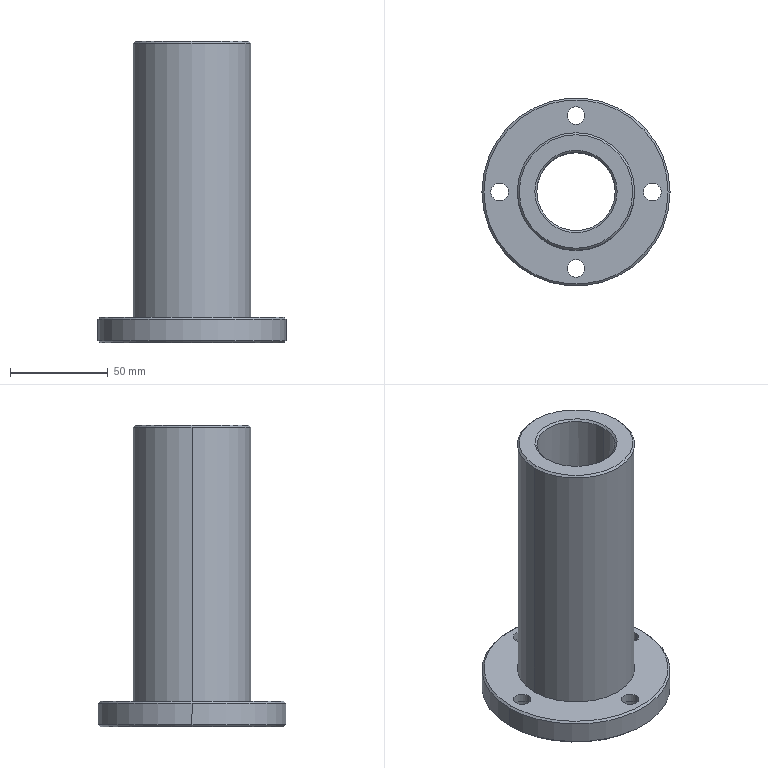Part | STEP file | LMF40LUU | 1 solid | 39 faces | box 96 x 96 x 154 mm | volume 291524 mm3 | cylinder 22 | cone 10 | plane 7 | commonest cylinder face diameters 9 x8 15 x8 40 x2 60 x2 96 x2